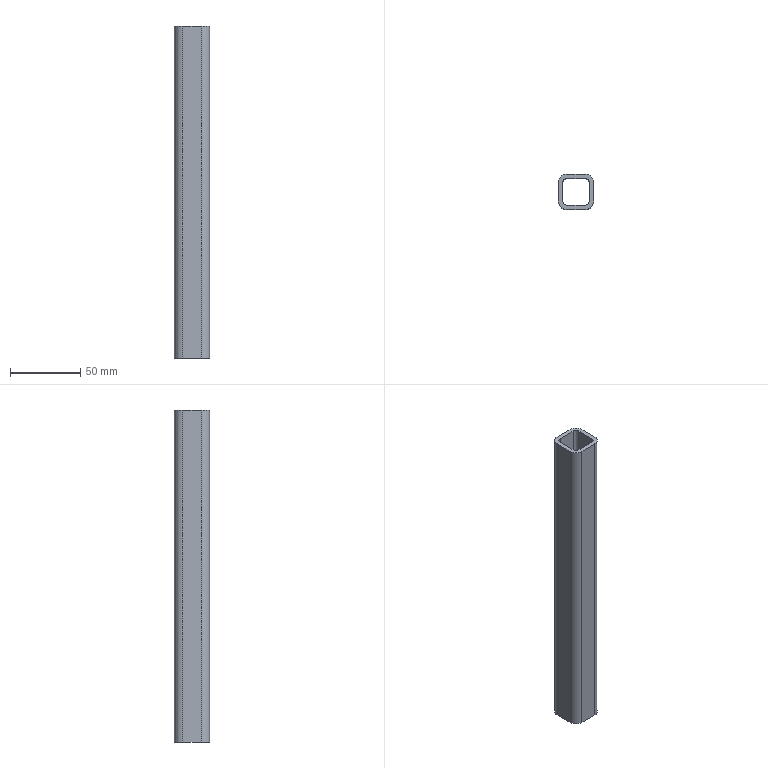Part | STEP file | ISO 10799-2 25x25x3 1784905468546 | 1 solid | 18 faces | box 25 x 25 x 236 mm | volume 56834 mm3 | plane 10 | cylinder 8 | commonest cylinder face diameters 6 x4 12 x4
STEP:
#1=CARTESIAN_POINT('',(-6.5,-9.5,261.));
#2=VERTEX_POINT('',#1);
#3=CARTESIAN_POINT('',(6.5,-9.5,261.));
#4=VERTEX_POINT('',#3);
#5=CARTESIAN_POINT('',(3.25,-9.5,261.));
#6=DIRECTION('',(1.,0.,0.));
#7=VECTOR('',#6,10.);
#8=LINE('',#5,#7);
#9=EDGE_CURVE('',#2,#4,#8,.T.);
#10=ORIENTED_EDGE('',*,*,#9,.T.);
#11=CARTESIAN_POINT('',(6.5,-9.5,25.));
#12=VERTEX_POINT('',#11);
#13=CARTESIAN_POINT('',(6.5,-9.5,0.));
#14=DIRECTION('',(0.,0.,1.));
#15=VECTOR('',#14,10.);
#16=LINE('',#13,#15);
#17=EDGE_CURVE('',#12,#4,#16,.T.);
#18=ORIENTED_EDGE('',*,*,#17,.F.);
#19=CARTESIAN_POINT('',(-6.5,-9.5,25.));
#20=VERTEX_POINT('',#19);
#21=CARTESIAN_POINT('',(3.25,-9.5,25.));
#22=DIRECTION('',(1.,0.,0.));
#23=VECTOR('',#22,10.);
#24=LINE('',#21,#23);
#25=EDGE_CURVE('',#20,#12,#24,.T.);
#26=ORIENTED_EDGE('',*,*,#25,.F.);
#27=CARTESIAN_POINT('',(-6.5,-9.5,0.));
#28=DIRECTION('',(0.,0.,1.));
#29=VECTOR('',#28,10.);
#30=LINE('',#27,#29);
#31=EDGE_CURVE('',#20,#2,#30,.T.);
#32=ORIENTED_EDGE('',*,*,#31,.T.);
#33=EDGE_LOOP('',(#10,#18,#26,#32));
#34=FACE_OUTER_BOUND('',#33,.T.);
#35=CARTESIAN_POINT('',(6.5,-9.5,0.));
#36=DIRECTION('',(0.,-1.,0.));
#37=DIRECTION('',(0.,0.,-1.));
#38=AXIS2_PLACEMENT_3D('',#35,#36,#37);
#39=PLANE('',#38);
#40=ADVANCED_FACE('',(#34),#39,.F.);
#41=CARTESIAN_POINT('',(9.5,-6.5,261.));
#42=VERTEX_POINT('',#41);
#43=CARTESIAN_POINT('',(6.5,-6.5,261.));
#44=DIRECTION('',(0.,0.,1.));
#45=DIRECTION('',(0.,1.,0.));
#46=AXIS2_PLACEMENT_3D('',#43,#44,#45);
#47=CIRCLE('',#46,3.);
#48=EDGE_CURVE('',#4,#42,#47,.T.);
#49=ORIENTED_EDGE('',*,*,#48,.T.);
#50=CARTESIAN_POINT('',(9.5,-6.5,25.));
#51=VERTEX_POINT('',#50);
#52=CARTESIAN_POINT('',(9.5,-6.5,0.));
#53=DIRECTION('',(0.,0.,1.));
#54=VECTOR('',#53,10.);
#55=LINE('',#52,#54);
#56=EDGE_CURVE('',#51,#42,#55,.T.);
#57=ORIENTED_EDGE('',*,*,#56,.F.);
#58=CARTESIAN_POINT('',(6.5,-6.5,25.));
#59=DIRECTION('',(0.,0.,1.));
#60=DIRECTION('',(0.,1.,0.));
#61=AXIS2_PLACEMENT_3D('',#58,#59,#60);
#62=CIRCLE('',#61,3.);
#63=EDGE_CURVE('',#12,#51,#62,.T.);
#64=ORIENTED_EDGE('',*,*,#63,.F.);
#65=ORIENTED_EDGE('',*,*,#17,.T.);
#66=EDGE_LOOP('',(#49,#57,#64,#65));
#67=FACE_OUTER_BOUND('',#66,.T.);
#68=CARTESIAN_POINT('',(6.5,-6.5,0.));
#69=DIRECTION('',(0.,0.,1.));
#70=DIRECTION('',(0.,1.,0.));
#71=AXIS2_PLACEMENT_3D('',#68,#69,#70);
#72=CYLINDRICAL_SURFACE('',#71,3.);
#73=ADVANCED_FACE('',(#67),#72,.F.);
#74=CARTESIAN_POINT('',(9.5,6.5,261.));
#75=VERTEX_POINT('',#74);
#76=CARTESIAN_POINT('',(9.5,3.25,261.));
#77=DIRECTION('',(0.,1.,0.));
#78=VECTOR('',#77,10.);
#79=LINE('',#76,#78);
#80=EDGE_CURVE('',#42,#75,#79,.T.);
#81=ORIENTED_EDGE('',*,*,#80,.T.);
#82=CARTESIAN_POINT('',(9.5,6.5,25.));
#83=VERTEX_POINT('',#82);
#84=CARTESIAN_POINT('',(9.5,6.5,0.));
#85=DIRECTION('',(0.,0.,1.));
#86=VECTOR('',#85,10.);
#87=LINE('',#84,#86);
#88=EDGE_CURVE('',#83,#75,#87,.T.);
#89=ORIENTED_EDGE('',*,*,#88,.F.);
#90=CARTESIAN_POINT('',(9.5,3.25,25.));
#91=DIRECTION('',(0.,1.,0.));
#92=VECTOR('',#91,10.);
#93=LINE('',#90,#92);
#94=EDGE_CURVE('',#51,#83,#93,.T.);
#95=ORIENTED_EDGE('',*,*,#94,.F.);
#96=ORIENTED_EDGE('',*,*,#56,.T.);
#97=EDGE_LOOP('',(#81,#89,#95,#96));
#98=FACE_OUTER_BOUND('',#97,.T.);
#99=CARTESIAN_POINT('',(9.5,6.5,0.));
#100=DIRECTION('',(1.,0.,0.));
#101=DIRECTION('',(0.,0.,-1.));
#102=AXIS2_PLACEMENT_3D('',#99,#100,#101);
#103=PLANE('',#102);
#104=ADVANCED_FACE('',(#98),#103,.F.);
#105=CARTESIAN_POINT('',(6.5,9.5,261.));
#106=VERTEX_POINT('',#105);
#107=CARTESIAN_POINT('',(6.5,6.5,261.));
#108=DIRECTION('',(0.,0.,1.));
#109=DIRECTION('',(-1.,0.,0.));
#110=AXIS2_PLACEMENT_3D('',#107,#108,#109);
#111=CIRCLE('',#110,3.);
#112=EDGE_CURVE('',#75,#106,#111,.T.);
#113=ORIENTED_EDGE('',*,*,#112,.T.);
#114=CARTESIAN_POINT('',(6.5,9.5,25.));
#115=VERTEX_POINT('',#114);
#116=CARTESIAN_POINT('',(6.5,9.5,0.));
#117=DIRECTION('',(0.,0.,1.));
#118=VECTOR('',#117,10.);
#119=LINE('',#116,#118);
#120=EDGE_CURVE('',#115,#106,#119,.T.);
#121=ORIENTED_EDGE('',*,*,#120,.F.);
#122=CARTESIAN_POINT('',(6.5,6.5,25.));
#123=DIRECTION('',(0.,0.,1.));
#124=DIRECTION('',(-1.,0.,0.));
#125=AXIS2_PLACEMENT_3D('',#122,#123,#124);
#126=CIRCLE('',#125,3.);
#127=EDGE_CURVE('',#83,#115,#126,.T.);
#128=ORIENTED_EDGE('',*,*,#127,.F.);
#129=ORIENTED_EDGE('',*,*,#88,.T.);
#130=EDGE_LOOP('',(#113,#121,#128,#129));
#131=FACE_OUTER_BOUND('',#130,.T.);
#132=CARTESIAN_POINT('',(6.5,6.5,0.));
#133=DIRECTION('',(0.,0.,1.));
#134=DIRECTION('',(-1.,0.,0.));
#135=AXIS2_PLACEMENT_3D('',#132,#133,#134);
#136=CYLINDRICAL_SURFACE('',#135,3.);
#137=ADVANCED_FACE('',(#131),#136,.F.);
#138=CARTESIAN_POINT('',(12.5,6.5,261.));
#139=VERTEX_POINT('',#138);
#140=CARTESIAN_POINT('',(12.5,-6.5,261.));
#141=VERTEX_POINT('',#140);
#142=CARTESIAN_POINT('',(12.5,3.25,261.));
#143=DIRECTION('',(0.,-1.,0.));
#144=VECTOR('',#143,10.);
#145=LINE('',#142,#144);
#146=EDGE_CURVE('',#139,#141,#145,.T.);
#147=ORIENTED_EDGE('',*,*,#146,.T.);
#148=CARTESIAN_POINT('',(12.5,-6.5,25.));
#149=VERTEX_POINT('',#148);
#150=CARTESIAN_POINT('',(12.5,-6.5,0.));
#151=DIRECTION('',(0.,0.,1.));
#152=VECTOR('',#151,10.);
#153=LINE('',#150,#152);
#154=EDGE_CURVE('',#149,#141,#153,.T.);
#155=ORIENTED_EDGE('',*,*,#154,.F.);
#156=CARTESIAN_POINT('',(12.5,6.5,25.));
#157=VERTEX_POINT('',#156);
#158=CARTESIAN_POINT('',(12.5,3.25,25.));
#159=DIRECTION('',(0.,-1.,0.));
#160=VECTOR('',#159,10.);
#161=LINE('',#158,#160);
#162=EDGE_CURVE('',#157,#149,#161,.T.);
#163=ORIENTED_EDGE('',*,*,#162,.F.);
#164=CARTESIAN_POINT('',(12.5,6.5,0.));
#165=DIRECTION('',(0.,0.,1.));
#166=VECTOR('',#165,10.);
#167=LINE('',#164,#166);
#168=EDGE_CURVE('',#157,#139,#167,.T.);
#169=ORIENTED_EDGE('',*,*,#168,.T.);
#170=EDGE_LOOP('',(#147,#155,#163,#169));
#171=FACE_OUTER_BOUND('',#170,.T.);
#172=CARTESIAN_POINT('',(12.5,6.5,0.));
#173=DIRECTION('',(1.,0.,0.));
#174=DIRECTION('',(0.,0.,-1.));
#175=AXIS2_PLACEMENT_3D('',#172,#173,#174);
#176=PLANE('',#175);
#177=ADVANCED_FACE('',(#171),#176,.T.);
#178=CARTESIAN_POINT('',(6.5,-12.5,261.));
#179=VERTEX_POINT('',#178);
#180=CARTESIAN_POINT('',(6.5,-6.5,261.));
#181=DIRECTION('',(0.,0.,-1.));
#182=DIRECTION('',(0.,1.,0.));
#183=AXIS2_PLACEMENT_3D('',#180,#181,#182);
#184=CIRCLE('',#183,6.);
#185=EDGE_CURVE('',#141,#179,#184,.T.);
#186=ORIENTED_EDGE('',*,*,#185,.T.);
#187=CARTESIAN_POINT('',(6.5,-12.5,25.));
#188=VERTEX_POINT('',#187);
#189=CARTESIAN_POINT('',(6.5,-12.5,0.));
#190=DIRECTION('',(0.,0.,1.));
#191=VECTOR('',#190,10.);
#192=LINE('',#189,#191);
#193=EDGE_CURVE('',#188,#179,#192,.T.);
#194=ORIENTED_EDGE('',*,*,#193,.F.);
#195=CARTESIAN_POINT('',(6.5,-6.5,25.));
#196=DIRECTION('',(0.,0.,-1.));
#197=DIRECTION('',(0.,1.,0.));
#198=AXIS2_PLACEMENT_3D('',#195,#196,#197);
#199=CIRCLE('',#198,6.);
#200=EDGE_CURVE('',#149,#188,#199,.T.);
#201=ORIENTED_EDGE('',*,*,#200,.F.);
#202=ORIENTED_EDGE('',*,*,#154,.T.);
#203=EDGE_LOOP('',(#186,#194,#201,#202));
#204=FACE_OUTER_BOUND('',#203,.T.);
#205=CARTESIAN_POINT('',(6.5,-6.5,0.));
#206=DIRECTION('',(0.,0.,1.));
#207=DIRECTION('',(0.,1.,0.));
#208=AXIS2_PLACEMENT_3D('',#205,#206,#207);
#209=CYLINDRICAL_SURFACE('',#208,6.);
#210=ADVANCED_FACE('',(#204),#209,.T.);
#211=CARTESIAN_POINT('',(-6.5,-12.5,261.));
#212=VERTEX_POINT('',#211);
#213=CARTESIAN_POINT('',(3.25,-12.5,261.));
#214=DIRECTION('',(-1.,0.,0.));
#215=VECTOR('',#214,10.);
#216=LINE('',#213,#215);
#217=EDGE_CURVE('',#179,#212,#216,.T.);
#218=ORIENTED_EDGE('',*,*,#217,.T.);
#219=CARTESIAN_POINT('',(-6.5,-12.5,25.));
#220=VERTEX_POINT('',#219);
#221=CARTESIAN_POINT('',(-6.5,-12.5,0.));
#222=DIRECTION('',(0.,0.,1.));
#223=VECTOR('',#222,10.);
#224=LINE('',#221,#223);
#225=EDGE_CURVE('',#220,#212,#224,.T.);
#226=ORIENTED_EDGE('',*,*,#225,.F.);
#227=CARTESIAN_POINT('',(3.25,-12.5,25.));
#228=DIRECTION('',(-1.,0.,0.));
#229=VECTOR('',#228,10.);
#230=LINE('',#227,#229);
#231=EDGE_CURVE('',#188,#220,#230,.T.);
#232=ORIENTED_EDGE('',*,*,#231,.F.);
#233=ORIENTED_EDGE('',*,*,#193,.T.);
#234=EDGE_LOOP('',(#218,#226,#232,#233));
#235=FACE_OUTER_BOUND('',#234,.T.);
#236=CARTESIAN_POINT('',(6.5,-12.5,0.));
#237=DIRECTION('',(0.,-1.,0.));
#238=DIRECTION('',(0.,0.,-1.));
#239=AXIS2_PLACEMENT_3D('',#236,#237,#238);
#240=PLANE('',#239);
#241=ADVANCED_FACE('',(#235),#240,.T.);
#242=CARTESIAN_POINT('',(-12.5,-6.5,261.));
#243=VERTEX_POINT('',#242);
#244=CARTESIAN_POINT('',(-6.5,-6.5,261.));
#245=DIRECTION('',(0.,0.,-1.));
#246=DIRECTION('',(1.,0.,0.));
#247=AXIS2_PLACEMENT_3D('',#244,#245,#246);
#248=CIRCLE('',#247,6.);
#249=EDGE_CURVE('',#212,#243,#248,.T.);
#250=ORIENTED_EDGE('',*,*,#249,.T.);
#251=CARTESIAN_POINT('',(-12.5,-6.5,25.));
#252=VERTEX_POINT('',#251);
#253=CARTESIAN_POINT('',(-12.5,-6.5,0.));
#254=DIRECTION('',(0.,0.,1.));
#255=VECTOR('',#254,10.);
#256=LINE('',#253,#255);
#257=EDGE_CURVE('',#252,#243,#256,.T.);
#258=ORIENTED_EDGE('',*,*,#257,.F.);
#259=CARTESIAN_POINT('',(-6.5,-6.5,25.));
#260=DIRECTION('',(0.,0.,-1.));
#261=DIRECTION('',(1.,0.,0.));
#262=AXIS2_PLACEMENT_3D('',#259,#260,#261);
#263=CIRCLE('',#262,6.);
#264=EDGE_CURVE('',#220,#252,#263,.T.);
#265=ORIENTED_EDGE('',*,*,#264,.F.);
#266=ORIENTED_EDGE('',*,*,#225,.T.);
#267=EDGE_LOOP('',(#250,#258,#265,#266));
#268=FACE_OUTER_BOUND('',#267,.T.);
#269=CARTESIAN_POINT('',(-6.5,-6.5,0.));
#270=DIRECTION('',(0.,0.,1.));
#271=DIRECTION('',(1.,0.,0.));
#272=AXIS2_PLACEMENT_3D('',#269,#270,#271);
#273=CYLINDRICAL_SURFACE('',#272,6.);
#274=ADVANCED_FACE('',(#268),#273,.T.);
#275=CARTESIAN_POINT('',(-6.5,9.5,261.));
#276=VERTEX_POINT('',#275);
#277=CARTESIAN_POINT('',(-3.25,9.5,261.));
#278=DIRECTION('',(-1.,0.,0.));
#279=VECTOR('',#278,10.);
#280=LINE('',#277,#279);
#281=EDGE_CURVE('',#106,#276,#280,.T.);
#282=ORIENTED_EDGE('',*,*,#281,.T.);
#283=CARTESIAN_POINT('',(-6.5,9.5,25.));
#284=VERTEX_POINT('',#283);
#285=CARTESIAN_POINT('',(-6.5,9.5,0.));
#286=DIRECTION('',(0.,0.,1.));
#287=VECTOR('',#286,10.);
#288=LINE('',#285,#287);
#289=EDGE_CURVE('',#284,#276,#288,.T.);
#290=ORIENTED_EDGE('',*,*,#289,.F.);
#291=CARTESIAN_POINT('',(-3.25,9.5,25.));
#292=DIRECTION('',(-1.,0.,0.));
#293=VECTOR('',#292,10.);
#294=LINE('',#291,#293);
#295=EDGE_CURVE('',#115,#284,#294,.T.);
#296=ORIENTED_EDGE('',*,*,#295,.F.);
#297=ORIENTED_EDGE('',*,*,#120,.T.);
#298=EDGE_LOOP('',(#282,#290,#296,#297));
#299=FACE_OUTER_BOUND('',#298,.T.);
#300=CARTESIAN_POINT('',(-6.5,9.5,0.));
#301=DIRECTION('',(0.,1.,0.));
#302=DIRECTION('',(0.,0.,1.));
#303=AXIS2_PLACEMENT_3D('',#300,#301,#302);
#304=PLANE('',#303);
#305=ADVANCED_FACE('',(#299),#304,.F.);
#306=CARTESIAN_POINT('',(-9.5,-6.5,261.));
#307=VERTEX_POINT('',#306);
#308=CARTESIAN_POINT('',(-6.5,-6.5,261.));
#309=DIRECTION('',(0.,0.,1.));
#310=DIRECTION('',(1.,0.,0.));
#311=AXIS2_PLACEMENT_3D('',#308,#309,#310);
#312=CIRCLE('',#311,3.);
#313=EDGE_CURVE('',#307,#2,#312,.T.);
#314=ORIENTED_EDGE('',*,*,#313,.T.);
#315=ORIENTED_EDGE('',*,*,#31,.F.);
#316=CARTESIAN_POINT('',(-9.5,-6.5,25.));
#317=VERTEX_POINT('',#316);
#318=CARTESIAN_POINT('',(-6.5,-6.5,25.));
#319=DIRECTION('',(0.,0.,1.));
#320=DIRECTION('',(1.,0.,0.));
#321=AXIS2_PLACEMENT_3D('',#318,#319,#320);
#322=CIRCLE('',#321,3.);
#323=EDGE_CURVE('',#317,#20,#322,.T.);
#324=ORIENTED_EDGE('',*,*,#323,.F.);
#325=CARTESIAN_POINT('',(-9.5,-6.5,0.));
#326=DIRECTION('',(0.,0.,1.));
#327=VECTOR('',#326,10.);
#328=LINE('',#325,#327);
#329=EDGE_CURVE('',#317,#307,#328,.T.);
#330=ORIENTED_EDGE('',*,*,#329,.T.);
#331=EDGE_LOOP('',(#314,#315,#324,#330));
#332=FACE_OUTER_BOUND('',#331,.T.);
#333=CARTESIAN_POINT('',(-6.5,-6.5,0.));
#334=DIRECTION('',(0.,0.,1.));
#335=DIRECTION('',(1.,0.,0.));
#336=AXIS2_PLACEMENT_3D('',#333,#334,#335);
#337=CYLINDRICAL_SURFACE('',#336,3.);
#338=ADVANCED_FACE('',(#332),#337,.F.);
#339=CARTESIAN_POINT('',(-9.5,6.5,261.));
#340=VERTEX_POINT('',#339);
#341=CARTESIAN_POINT('',(-9.5,-3.25,261.));
#342=DIRECTION('',(0.,-1.,0.));
#343=VECTOR('',#342,10.);
#344=LINE('',#341,#343);
#345=EDGE_CURVE('',#340,#307,#344,.T.);
#346=ORIENTED_EDGE('',*,*,#345,.T.);
#347=ORIENTED_EDGE('',*,*,#329,.F.);
#348=CARTESIAN_POINT('',(-9.5,6.5,25.));
#349=VERTEX_POINT('',#348);
#350=CARTESIAN_POINT('',(-9.5,-3.25,25.));
#351=DIRECTION('',(0.,-1.,0.));
#352=VECTOR('',#351,10.);
#353=LINE('',#350,#352);
#354=EDGE_CURVE('',#349,#317,#353,.T.);
#355=ORIENTED_EDGE('',*,*,#354,.F.);
#356=CARTESIAN_POINT('',(-9.5,6.5,0.));
#357=DIRECTION('',(0.,0.,1.));
#358=VECTOR('',#357,10.);
#359=LINE('',#356,#358);
#360=EDGE_CURVE('',#349,#340,#359,.T.);
#361=ORIENTED_EDGE('',*,*,#360,.T.);
#362=EDGE_LOOP('',(#346,#347,#355,#361));
#363=FACE_OUTER_BOUND('',#362,.T.);
#364=CARTESIAN_POINT('',(-9.5,-6.5,0.));
#365=DIRECTION('',(-1.,0.,0.));
#366=DIRECTION('',(0.,0.,1.));
#367=AXIS2_PLACEMENT_3D('',#364,#365,#366);
#368=PLANE('',#367);
#369=ADVANCED_FACE('',(#363),#368,.F.);
#370=CARTESIAN_POINT('',(-6.5,6.5,261.));
#371=DIRECTION('',(0.,0.,1.));
#372=DIRECTION('',(0.,-1.,0.));
#373=AXIS2_PLACEMENT_3D('',#370,#371,#372);
#374=CIRCLE('',#373,3.);
#375=EDGE_CURVE('',#276,#340,#374,.T.);
#376=ORIENTED_EDGE('',*,*,#375,.T.);
#377=ORIENTED_EDGE('',*,*,#360,.F.);
#378=CARTESIAN_POINT('',(-6.5,6.5,25.));
#379=DIRECTION('',(0.,0.,1.));
#380=DIRECTION('',(0.,-1.,0.));
#381=AXIS2_PLACEMENT_3D('',#378,#379,#380);
#382=CIRCLE('',#381,3.);
#383=EDGE_CURVE('',#284,#349,#382,.T.);
#384=ORIENTED_EDGE('',*,*,#383,.F.);
#385=ORIENTED_EDGE('',*,*,#289,.T.);
#386=EDGE_LOOP('',(#376,#377,#384,#385));
#387=FACE_OUTER_BOUND('',#386,.T.);
#388=CARTESIAN_POINT('',(-6.5,6.5,0.));
#389=DIRECTION('',(0.,0.,1.));
#390=DIRECTION('',(0.,-1.,0.));
#391=AXIS2_PLACEMENT_3D('',#388,#389,#390);
#392=CYLINDRICAL_SURFACE('',#391,3.);
#393=ADVANCED_FACE('',(#387),#392,.F.);
#394=CARTESIAN_POINT('',(-12.5,6.5,261.));
#395=VERTEX_POINT('',#394);
#396=CARTESIAN_POINT('',(-12.5,-3.25,261.));
#397=DIRECTION('',(0.,1.,0.));
#398=VECTOR('',#397,10.);
#399=LINE('',#396,#398);
#400=EDGE_CURVE('',#243,#395,#399,.T.);
#401=ORIENTED_EDGE('',*,*,#400,.T.);
#402=CARTESIAN_POINT('',(-12.5,6.5,25.));
#403=VERTEX_POINT('',#402);
#404=CARTESIAN_POINT('',(-12.5,6.5,0.));
#405=DIRECTION('',(0.,0.,1.));
#406=VECTOR('',#405,10.);
#407=LINE('',#404,#406);
#408=EDGE_CURVE('',#403,#395,#407,.T.);
#409=ORIENTED_EDGE('',*,*,#408,.F.);
#410=CARTESIAN_POINT('',(-12.5,-3.25,25.));
#411=DIRECTION('',(0.,1.,0.));
#412=VECTOR('',#411,10.);
#413=LINE('',#410,#412);
#414=EDGE_CURVE('',#252,#403,#413,.T.);
#415=ORIENTED_EDGE('',*,*,#414,.F.);
#416=ORIENTED_EDGE('',*,*,#257,.T.);
#417=EDGE_LOOP('',(#401,#409,#415,#416));
#418=FACE_OUTER_BOUND('',#417,.T.);
#419=CARTESIAN_POINT('',(-12.5,-6.5,0.));
#420=DIRECTION('',(-1.,0.,0.));
#421=DIRECTION('',(0.,0.,1.));
#422=AXIS2_PLACEMENT_3D('',#419,#420,#421);
#423=PLANE('',#422);
#424=ADVANCED_FACE('',(#418),#423,.T.);
#425=CARTESIAN_POINT('',(-6.5,12.5,261.));
#426=VERTEX_POINT('',#425);
#427=CARTESIAN_POINT('',(-6.5,6.5,261.));
#428=DIRECTION('',(0.,0.,-1.));
#429=DIRECTION('',(0.,-1.,0.));
#430=AXIS2_PLACEMENT_3D('',#427,#428,#429);
#431=CIRCLE('',#430,6.);
#432=EDGE_CURVE('',#395,#426,#431,.T.);
#433=ORIENTED_EDGE('',*,*,#432,.T.);
#434=CARTESIAN_POINT('',(-6.5,12.5,25.));
#435=VERTEX_POINT('',#434);
#436=CARTESIAN_POINT('',(-6.5,12.5,0.));
#437=DIRECTION('',(0.,0.,1.));
#438=VECTOR('',#437,10.);
#439=LINE('',#436,#438);
#440=EDGE_CURVE('',#435,#426,#439,.T.);
#441=ORIENTED_EDGE('',*,*,#440,.F.);
#442=CARTESIAN_POINT('',(-6.5,6.5,25.));
#443=DIRECTION('',(0.,0.,-1.));
#444=DIRECTION('',(0.,-1.,0.));
#445=AXIS2_PLACEMENT_3D('',#442,#443,#444);
#446=CIRCLE('',#445,6.);
#447=EDGE_CURVE('',#403,#435,#446,.T.);
#448=ORIENTED_EDGE('',*,*,#447,.F.);
#449=ORIENTED_EDGE('',*,*,#408,.T.);
#450=EDGE_LOOP('',(#433,#441,#448,#449));
#451=FACE_OUTER_BOUND('',#450,.T.);
#452=CARTESIAN_POINT('',(-6.5,6.5,0.));
#453=DIRECTION('',(0.,0.,1.));
#454=DIRECTION('',(0.,-1.,0.));
#455=AXIS2_PLACEMENT_3D('',#452,#453,#454);
#456=CYLINDRICAL_SURFACE('',#455,6.);
#457=ADVANCED_FACE('',(#451),#456,.T.);
#458=CARTESIAN_POINT('',(6.5,12.5,261.));
#459=VERTEX_POINT('',#458);
#460=CARTESIAN_POINT('',(-3.25,12.5,261.));
#461=DIRECTION('',(1.,0.,0.));
#462=VECTOR('',#461,10.);
#463=LINE('',#460,#462);
#464=EDGE_CURVE('',#426,#459,#463,.T.);
#465=ORIENTED_EDGE('',*,*,#464,.T.);
#466=CARTESIAN_POINT('',(6.5,12.5,25.));
#467=VERTEX_POINT('',#466);
#468=CARTESIAN_POINT('',(6.5,12.5,0.));
#469=DIRECTION('',(0.,0.,1.));
#470=VECTOR('',#469,10.);
#471=LINE('',#468,#470);
#472=EDGE_CURVE('',#467,#459,#471,.T.);
#473=ORIENTED_EDGE('',*,*,#472,.F.);
#474=CARTESIAN_POINT('',(-3.25,12.5,25.));
#475=DIRECTION('',(1.,0.,0.));
#476=VECTOR('',#475,10.);
#477=LINE('',#474,#476);
#478=EDGE_CURVE('',#435,#467,#477,.T.);
#479=ORIENTED_EDGE('',*,*,#478,.F.);
#480=ORIENTED_EDGE('',*,*,#440,.T.);
#481=EDGE_LOOP('',(#465,#473,#479,#480));
#482=FACE_OUTER_BOUND('',#481,.T.);
#483=CARTESIAN_POINT('',(-6.5,12.5,0.));
#484=DIRECTION('',(0.,1.,0.));
#485=DIRECTION('',(0.,0.,1.));
#486=AXIS2_PLACEMENT_3D('',#483,#484,#485);
#487=PLANE('',#486);
#488=ADVANCED_FACE('',(#482),#487,.T.);
#489=CARTESIAN_POINT('',(6.5,6.5,261.));
#490=DIRECTION('',(0.,0.,-1.));
#491=DIRECTION('',(-1.,0.,0.));
#492=AXIS2_PLACEMENT_3D('',#489,#490,#491);
#493=CIRCLE('',#492,6.);
#494=EDGE_CURVE('',#459,#139,#493,.T.);
#495=ORIENTED_EDGE('',*,*,#494,.T.);
#496=ORIENTED_EDGE('',*,*,#168,.F.);
#497=CARTESIAN_POINT('',(6.5,6.5,25.));
#498=DIRECTION('',(0.,0.,-1.));
#499=DIRECTION('',(-1.,0.,0.));
#500=AXIS2_PLACEMENT_3D('',#497,#498,#499);
#501=CIRCLE('',#500,6.);
#502=EDGE_CURVE('',#467,#157,#501,.T.);
#503=ORIENTED_EDGE('',*,*,#502,.F.);
#504=ORIENTED_EDGE('',*,*,#472,.T.);
#505=EDGE_LOOP('',(#495,#496,#503,#504));
#506=FACE_OUTER_BOUND('',#505,.T.);
#507=CARTESIAN_POINT('',(6.5,6.5,0.));
#508=DIRECTION('',(0.,0.,1.));
#509=DIRECTION('',(-1.,0.,0.));
#510=AXIS2_PLACEMENT_3D('',#507,#508,#509);
#511=CYLINDRICAL_SURFACE('',#510,6.);
#512=ADVANCED_FACE('',(#506),#511,.T.);
#513=ORIENTED_EDGE('',*,*,#414,.T.);
#514=ORIENTED_EDGE('',*,*,#447,.T.);
#515=ORIENTED_EDGE('',*,*,#478,.T.);
#516=ORIENTED_EDGE('',*,*,#502,.T.);
#517=ORIENTED_EDGE('',*,*,#162,.T.);
#518=ORIENTED_EDGE('',*,*,#200,.T.);
#519=ORIENTED_EDGE('',*,*,#231,.T.);
#520=ORIENTED_EDGE('',*,*,#264,.T.);
#521=EDGE_LOOP('',(#513,#514,#515,#516,#517,#518,#519,#520));
#522=FACE_OUTER_BOUND('',#521,.T.);
#523=ORIENTED_EDGE('',*,*,#295,.T.);
#524=ORIENTED_EDGE('',*,*,#383,.T.);
#525=ORIENTED_EDGE('',*,*,#354,.T.);
#526=ORIENTED_EDGE('',*,*,#323,.T.);
#527=ORIENTED_EDGE('',*,*,#25,.T.);
#528=ORIENTED_EDGE('',*,*,#63,.T.);
#529=ORIENTED_EDGE('',*,*,#94,.T.);
#530=ORIENTED_EDGE('',*,*,#127,.T.);
#531=EDGE_LOOP('',(#523,#524,#525,#526,#527,#528,#529,#530));
#532=FACE_BOUND('',#531,.T.);
#533=CARTESIAN_POINT('',(0.,0.,25.));
#534=DIRECTION('',(0.,0.,1.));
#535=DIRECTION('',(1.,0.,0.));
#536=AXIS2_PLACEMENT_3D('',#533,#534,#535);
#537=PLANE('',#536);
#538=ADVANCED_FACE('',(#522,#532),#537,.F.);
#539=ORIENTED_EDGE('',*,*,#400,.F.);
#540=ORIENTED_EDGE('',*,*,#249,.F.);
#541=ORIENTED_EDGE('',*,*,#217,.F.);
#542=ORIENTED_EDGE('',*,*,#185,.F.);
#543=ORIENTED_EDGE('',*,*,#146,.F.);
#544=ORIENTED_EDGE('',*,*,#494,.F.);
#545=ORIENTED_EDGE('',*,*,#464,.F.);
#546=ORIENTED_EDGE('',*,*,#432,.F.);
#547=EDGE_LOOP('',(#539,#540,#541,#542,#543,#544,#545,#546));
#548=FACE_OUTER_BOUND('',#547,.T.);
#549=ORIENTED_EDGE('',*,*,#281,.F.);
#550=ORIENTED_EDGE('',*,*,#112,.F.);
#551=ORIENTED_EDGE('',*,*,#80,.F.);
#552=ORIENTED_EDGE('',*,*,#48,.F.);
#553=ORIENTED_EDGE('',*,*,#9,.F.);
#554=ORIENTED_EDGE('',*,*,#313,.F.);
#555=ORIENTED_EDGE('',*,*,#345,.F.);
#556=ORIENTED_EDGE('',*,*,#375,.F.);
#557=EDGE_LOOP('',(#549,#550,#551,#552,#553,#554,#555,#556));
#558=FACE_BOUND('',#557,.T.);
#559=CARTESIAN_POINT('',(0.,0.,261.));
#560=DIRECTION('',(0.,0.,1.));
#561=DIRECTION('',(1.,0.,0.));
#562=AXIS2_PLACEMENT_3D('',#559,#560,#561);
#563=PLANE('',#562);
#564=ADVANCED_FACE('',(#548,#558),#563,.T.);
#565=CLOSED_SHELL('',(#40,#73,#104,#137,#177,#210,#241,#274,#305,#338,#369,#393,#424,#457,#488,#512,#538,#564));
#566=MANIFOLD_SOLID_BREP('',#565);
#567=(LENGTH_UNIT()NAMED_UNIT(*)SI_UNIT(.MILLI.,.METRE.));
#568=UNCERTAINTY_MEASURE_WITH_UNIT(LENGTH_MEASURE(0.01),#567,'','');
#569=(NAMED_UNIT(*)PLANE_ANGLE_UNIT()SI_UNIT($,.RADIAN.));
#570=(NAMED_UNIT(*)SI_UNIT($,.STERADIAN.)SOLID_ANGLE_UNIT());
#571=(GEOMETRIC_REPRESENTATION_CONTEXT(3)GLOBAL_UNCERTAINTY_ASSIGNED_CONTEXT((#568))GLOBAL_UNIT_ASSIGNED_CONTEXT((#567,#569,#570))REPRESENTATION_CONTEXT('',''));
#572=ADVANCED_BREP_SHAPE_REPRESENTATION('',(#566),#571);